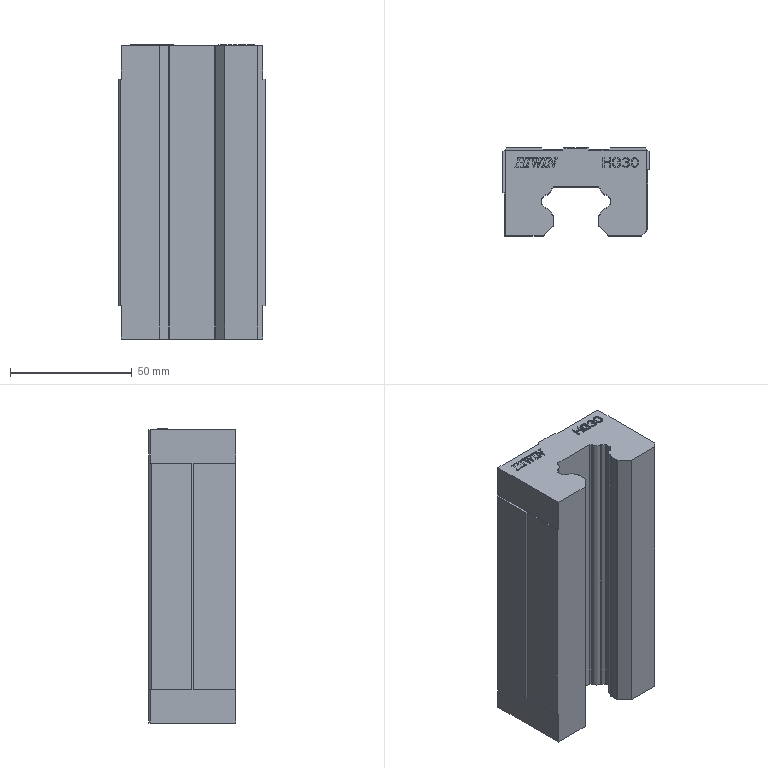Part | SolidWorks | features Draft 43, Chamfer 42, ICE 29, Fillet 8, BaseBody 1, HoleWzd 1 | 1 solid | 380 faces | box 60 x 36 x 120.7 mm | volume 197221 mm3 | plane 298 | spline 42 | cylinder 40 | commonest cylinder face diameters 1.2 x12 8 x8 1.6 x4 5.66 x4 0.462 x1 2.385 x1